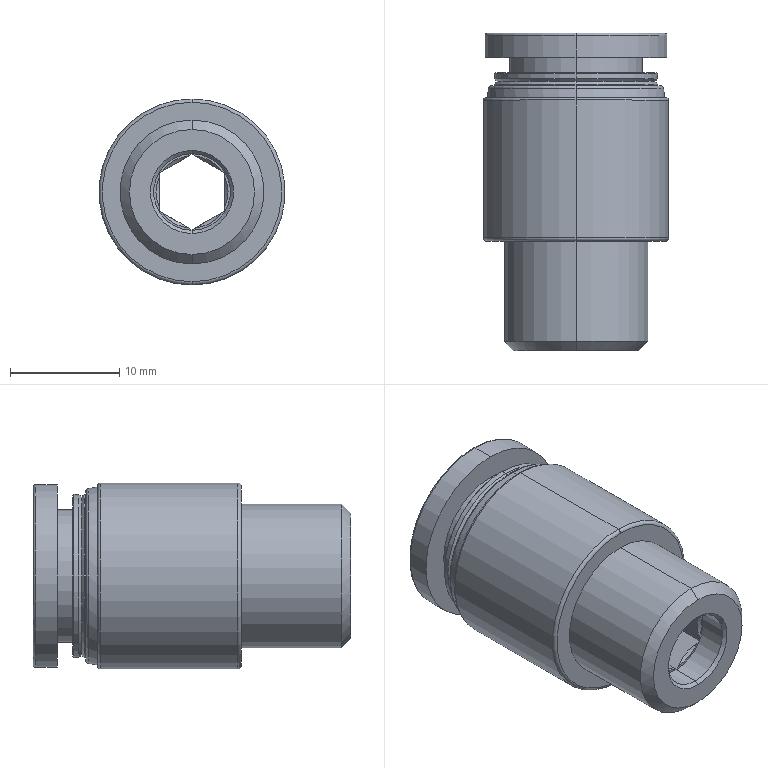Part | STEP file | POC1002D | 1 solid | 60 faces | box 17 x 29 x 17 mm | volume 3444 mm3 | cone 20 | cylinder 16 | plane 14 | torus 10 | commonest cylinder face diameters 14.9 x4 7 x2 10 x2 12.1 x2 13.157 x2 16.7 x2